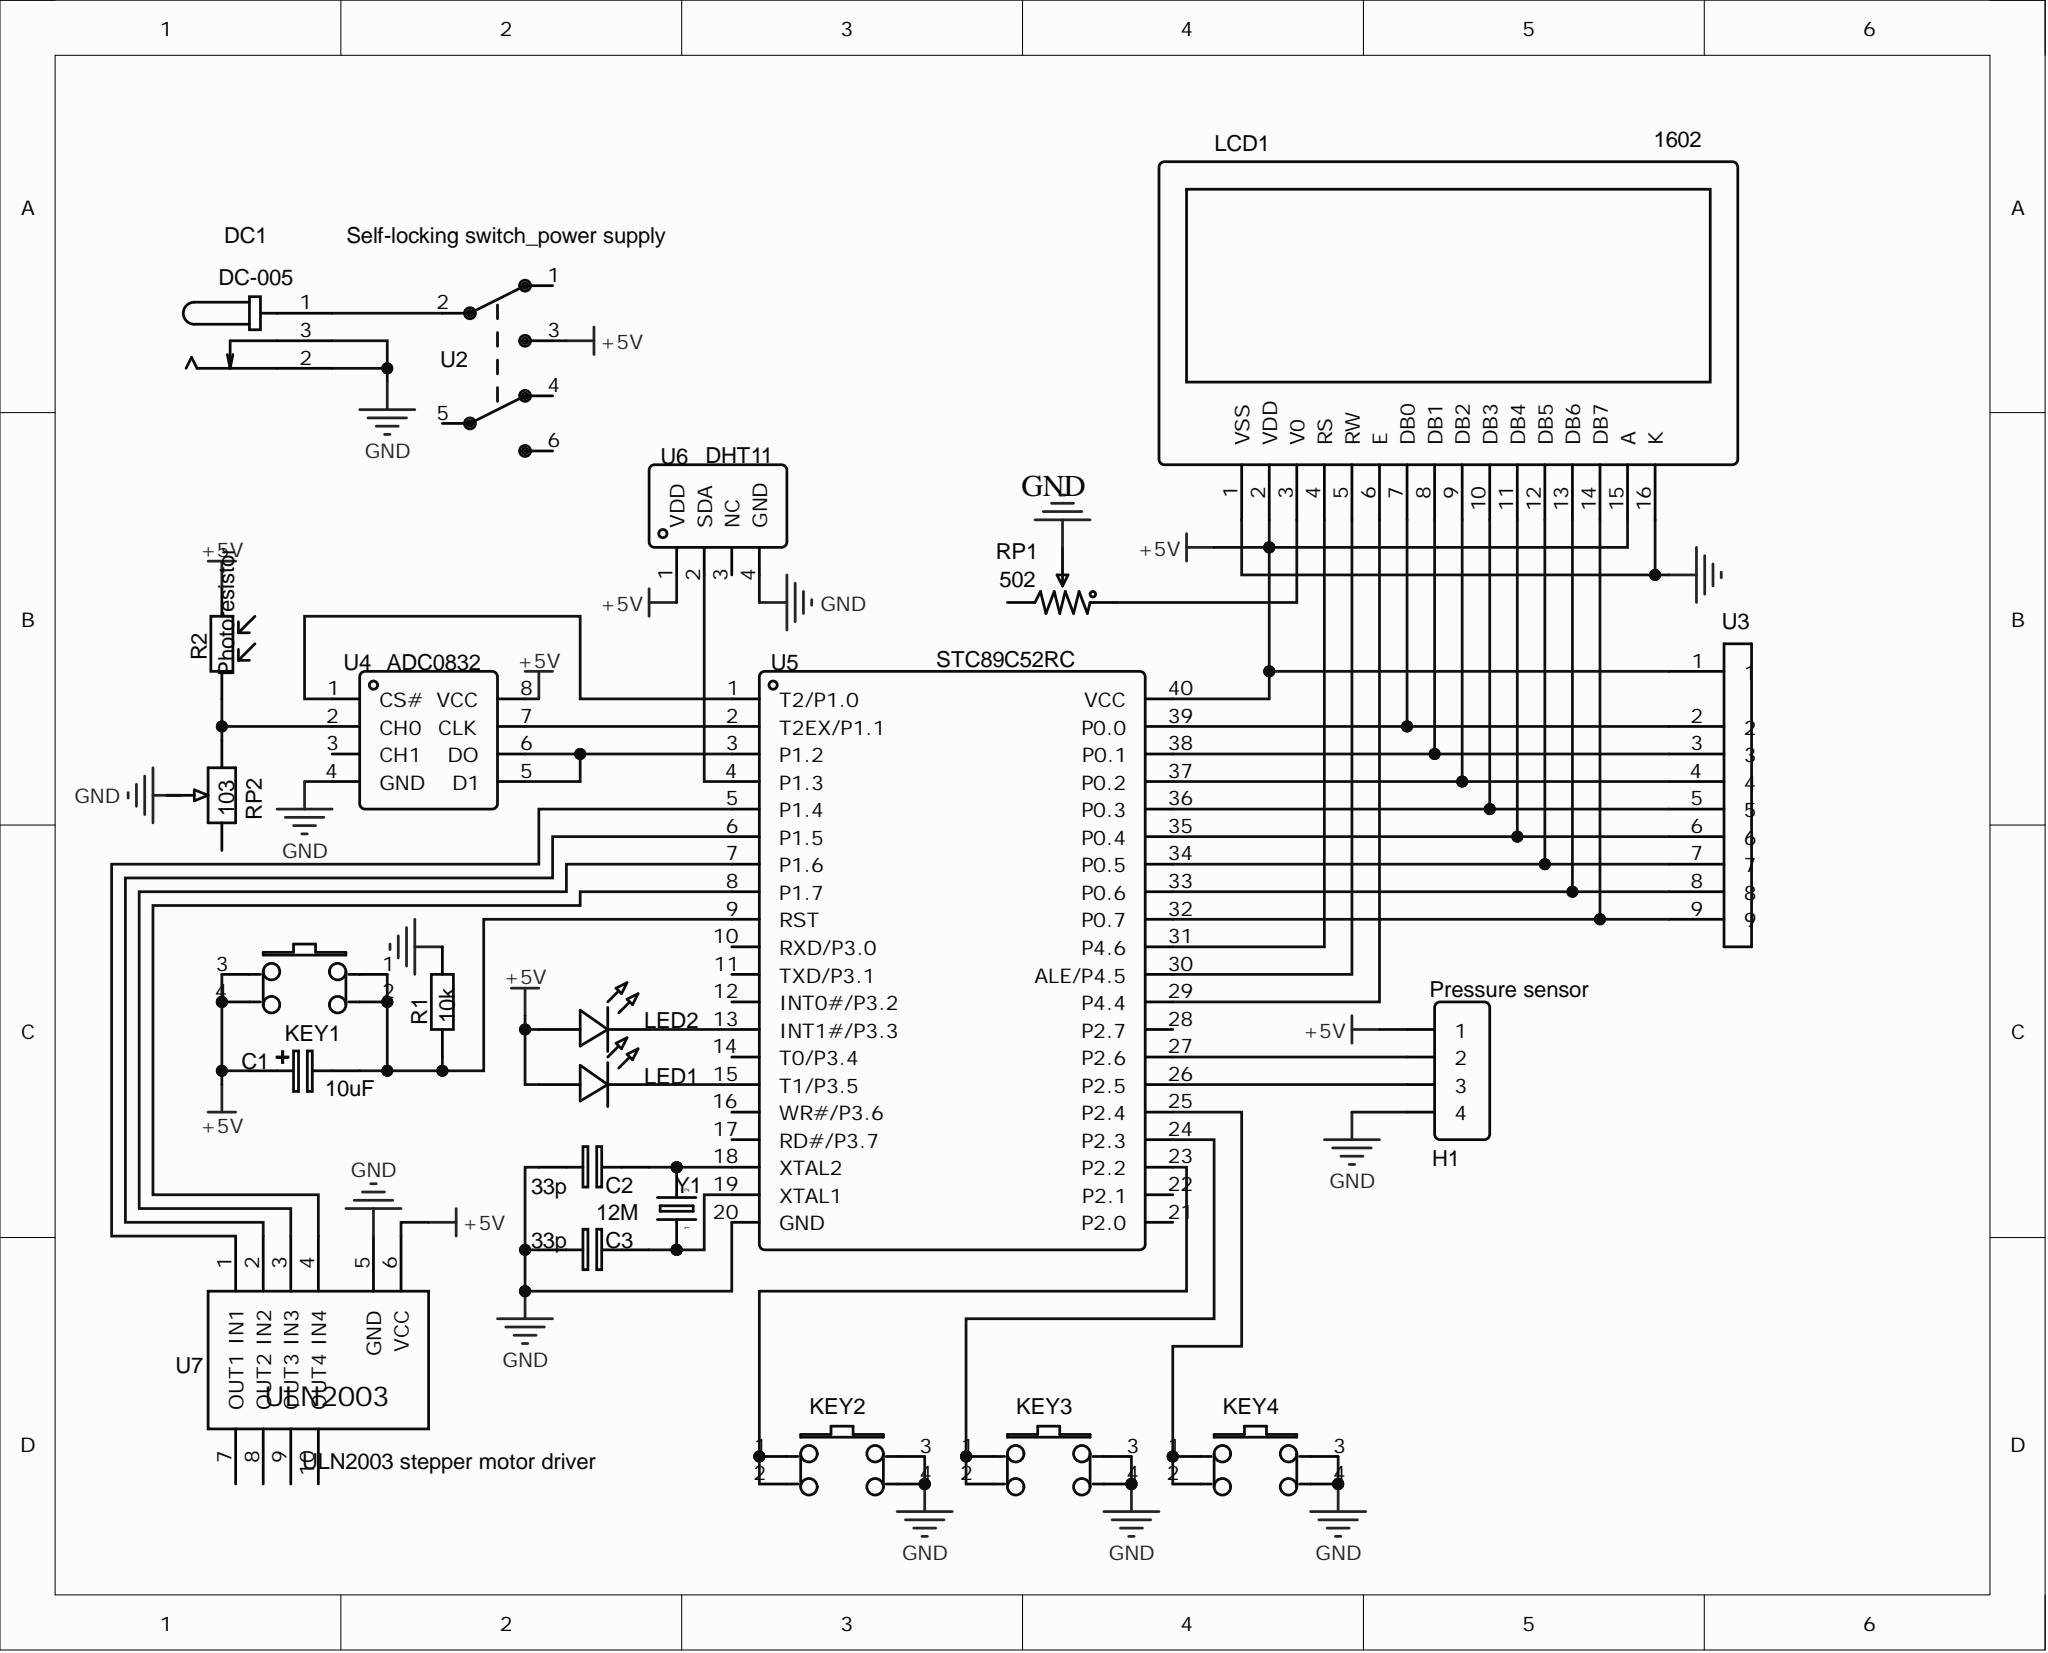Circuit board | Altium Designer | 23 parts | 34 nets
Bill of materials:
Comment,Description,Designator,Footprint,LibRef,Quantity
"10uF","","C1","RB7.6-15","10uF","1"
"33p","","C2, C3","RAD-0.1","33p","2"
"DC-005","","DC1","DC-005","DC-005","1"
"Pressure sensor","","H1","HDR1X4","气压传感器","1"
"button6*6*8.5","","KEY1, KEY2, KEY3, KEY4","四脚轻触开关","button6*6*8.5","4"
"LED-0603_R","","LED1, LED2","LED3MM","LED-0603_R","2"
"10k","","R1","AXIAL-0.3","10k","1"
"Photoresistor","","R2","AXIAL-0.6","光敏","1"
"502","","RP1","电位器","502","1"
"103","","RP2","RM065","103","1"
"1602","","U1","LCD1602","1602","1"
"Self-locking switch_power supply","","U2","自锁开关","自锁开关_电源供电","1"
"respack-8","","U3","HDR1X9","respack-8","1"
"ADC0832","","U4","DIP-8","ADC0832","1"
"STC89C52RC","","U5","DIP40","STC89C52RC","1"
"DHT11","","U6","HDR1X4","DHT11","1"
"ULN2003 stepper motor driver","","U7","ULN2003","ULN2003步进电机驱动","1"
"12M","","Y1","R38","12M","1"
Netlist (Protel format):
[
C1
RB7.6-15
10uF



]
[
C2
RAD-0.1
33p



]
[
C3
RAD-0.1
33p



]
[
DC1
DC-005
DC-005



]
[
H1
HDR1X4
Pressure sensor



]
[
KEY1
四脚轻触开关
button6*6*8.5



]
[
KEY2
四脚轻触开关
button6*6*8.5



]
[
KEY3
四脚轻触开关
button6*6*8.5



]
[
KEY4
四脚轻触开关
button6*6*8.5



]
[
LED1
LED3MM
LED-0603_R



]
[
LED2
LED3MM
LED-0603_R



]
[
R1
AXIAL-0.3
10k



]
[
R2
AXIAL-0.6
Photoresistor



]
[
RP1
电位器
502



]
[
RP2
RM065
103



]
[
U1
LCD1602
1602



]
[
U2
自锁开关
Self-locking switch_power supply



]
[
U3
HDR1X9
respack-8



]
[
U4
DIP-8
ADC0832



]
[
U5
DIP40
STC89C52RC



]
[
U6
HDR1X4
DHT11



]
[
U7
ULN2003
ULN2003 stepper motor driver



]
[
Y1
R38
12M



]
(
NetU5_8
U5-8
U7-4
)
(
NetU5_7
U5-7
U7-3
)
(
NetU5_6
U5-6
U7-2
)
(
NetU5_5
U5-5
U7-1
)
(
NetU5_4
U5-4
U6-2
)
(
NetU4_7
U4-7
U5-2
)
(
NetU4_5
U4-5
U4-6
U5-3
)
(
NetU4_1
U4-1
U5-1
)
(
NetU1_14
U1-14
U3-9
U5-32
)
(
NetU1_13
U1-13
U3-8
U5-33
)
(
NetU1_12
U1-12
U3-7
U5-34
)
(
NetU1_11
U1-11
U3-6
U5-35
)
(
NetU1_10
U1-10
U3-5
U5-36
)
(
NetU1_9
U1-9
U3-4
U5-37
)
(
NetU1_8
U1-8
U3-3
U5-38
)
(
NetU1_7
U1-7
U3-2
U5-39
)
(
NetU1_6
U1-6
U5-29
)
(
NetU1_5
U1-5
U5-30
)
(
NetU1_4
U1-4
U5-31
)
(
NetRP1_1
RP1-1
U1-3
)
(
NetR2_2
R2-2
RP2-3
U4-2
)
(
NetLED2_2
LED2-2
U5-15
)
(
NetLED1_2
LED1-2
U5-13
)
(
NetKEY4_1
KEY4-1
KEY4-2
U5-25
)
(
NetKEY3_1
KEY3-1
KEY3-2
U5-24
)
(
NetKEY2_1
KEY2-1
KEY2-2
U5-23
)
(
NetH1_3
H1-3
U5-26
)
(
NetH1_2
H1-2
U5-27
)
(
NetDC1_1
DC1-1
U2-2
)
(
NetC3_2
C3-2
U5-19
Y1-1
)
(
NetC2_2
C2-2
U5-18
Y1-2
)
(
NetC1_2
C1-2
KEY1-1
KEY1-2
R1-1
U5-9
)
(
GND
C2-1
C3-1
DC1-2
DC1-3
H1-4
KEY2-3
KEY2-4
KEY3-3
KEY3-4
KEY4-3
KEY4-4
R1-2
RP1-2
RP2-2
U1-1
U1-16
U4-4
U5-20
U6-4
U7-5
)
(
+5V
C1-1
H1-1
KEY1-3
KEY1-4
LED1-1
LED2-1
R2-1
U1-2
U1-15
U2-3
U3-1
U4-8
U5-40
U6-1
U7-6
)